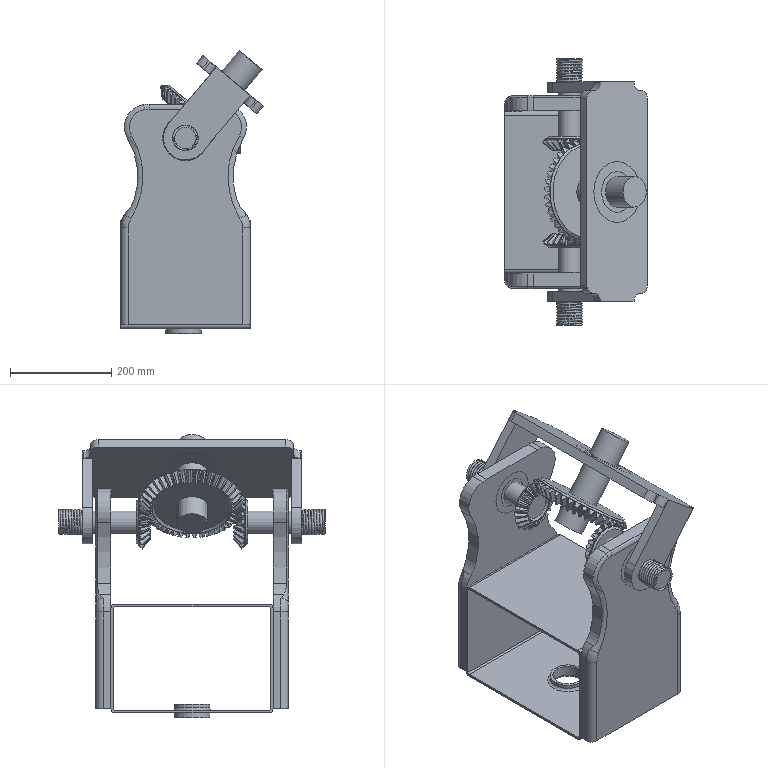Part | NX | features BREP 1 | 17 solids | 1291 faces | volume 10833655 mm3 | spline 730 | plane 309 | cone 166 | cylinder 68 | torus 18 | commonest cylinder face diameters 30 x14 60 x8 90 x8 45 x6 6 x4 16 x4